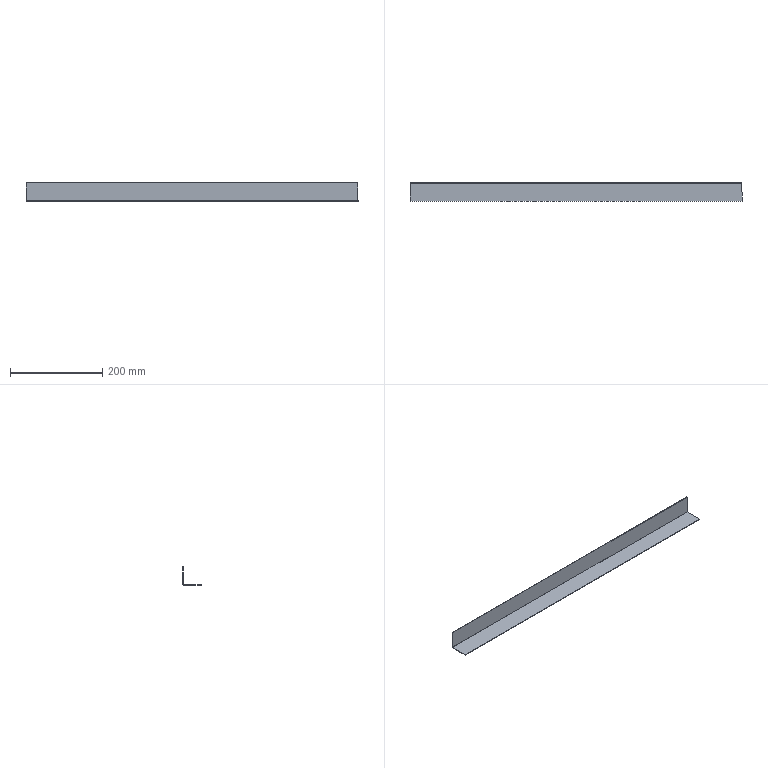Part | SolidWorks | features EdgeFlange 1, FlatPattern 1, SMBaseFlange 1, SheetMetal 1 | 1 solid | 14 faces | box 720 x 40 x 40 mm | volume 67824 mm3 | plane 12 | cylinder 2 | commonest cylinder face diameters 0.2 x1 2.6 x1
STEP:
#1=CARTESIAN_POINT('',(-360.,18.7,0.));
#2=VERTEX_POINT('',#1);
#3=CARTESIAN_POINT('',(-360.,-20.,0.));
#4=VERTEX_POINT('',#3);
#5=CARTESIAN_POINT('',(-360.,20.,0.));
#6=DIRECTION('',(0.,-1.,0.));
#7=VECTOR('',#6,1000.);
#8=LINE('',#5,#7);
#9=EDGE_CURVE('',#2,#4,#8,.T.);
#10=ORIENTED_EDGE('',*,*,#9,.F.);
#11=CARTESIAN_POINT('',(-360.,18.7,-1.2));
#12=VERTEX_POINT('',#11);
#13=CARTESIAN_POINT('',(-360.,18.7,0.));
#14=DIRECTION('',(0.,0.,-1.));
#15=VECTOR('',#14,1000.);
#16=LINE('',#13,#15);
#17=EDGE_CURVE('',#2,#12,#16,.T.);
#18=ORIENTED_EDGE('',*,*,#17,.T.);
#19=CARTESIAN_POINT('',(-360.,-20.,-1.2));
#20=VERTEX_POINT('',#19);
#21=CARTESIAN_POINT('',(-360.,20.,-1.2));
#22=DIRECTION('',(0.,-1.,0.));
#23=VECTOR('',#22,1000.);
#24=LINE('',#21,#23);
#25=EDGE_CURVE('',#12,#20,#24,.T.);
#26=ORIENTED_EDGE('',*,*,#25,.T.);
#27=CARTESIAN_POINT('',(-360.,-20.,-1.2));
#28=DIRECTION('',(0.,0.,1.));
#29=VECTOR('',#28,1000.);
#30=LINE('',#27,#29);
#31=EDGE_CURVE('',#20,#4,#30,.T.);
#32=ORIENTED_EDGE('',*,*,#31,.T.);
#33=EDGE_LOOP('',(#10,#18,#26,#32));
#34=FACE_OUTER_BOUND('',#33,.T.);
#35=CARTESIAN_POINT('',(-360.,20.,-1.2));
#36=DIRECTION('',(-1.,0.,0.));
#37=DIRECTION('',(0.,0.,1.));
#38=AXIS2_PLACEMENT_3D('',#35,#36,#37);
#39=PLANE('',#38);
#40=ADVANCED_FACE('',(#34),#39,.T.);
#41=CARTESIAN_POINT('',(360.,18.7,-1.2));
#42=VERTEX_POINT('',#41);
#43=CARTESIAN_POINT('',(-360.,18.7,-1.2));
#44=DIRECTION('',(1.,0.,0.));
#45=VECTOR('',#44,1000.);
#46=LINE('',#43,#45);
#47=EDGE_CURVE('',#12,#42,#46,.T.);
#48=ORIENTED_EDGE('',*,*,#47,.T.);
#49=CARTESIAN_POINT('',(360.,-20.,-1.2));
#50=VERTEX_POINT('',#49);
#51=CARTESIAN_POINT('',(360.,20.,-1.2));
#52=DIRECTION('',(0.,1.,0.));
#53=VECTOR('',#52,1000.);
#54=LINE('',#51,#53);
#55=EDGE_CURVE('',#50,#42,#54,.T.);
#56=ORIENTED_EDGE('',*,*,#55,.F.);
#57=CARTESIAN_POINT('',(-360.,-20.,-1.2));
#58=DIRECTION('',(1.,0.,0.));
#59=VECTOR('',#58,1000.);
#60=LINE('',#57,#59);
#61=EDGE_CURVE('',#20,#50,#60,.T.);
#62=ORIENTED_EDGE('',*,*,#61,.F.);
#63=ORIENTED_EDGE('',*,*,#25,.F.);
#64=EDGE_LOOP('',(#48,#56,#62,#63));
#65=FACE_OUTER_BOUND('',#64,.T.);
#66=CARTESIAN_POINT('',(0.,0.,-1.2));
#67=DIRECTION('',(0.,0.,1.));
#68=DIRECTION('',(1.,0.,0.));
#69=AXIS2_PLACEMENT_3D('',#66,#67,#68);
#70=PLANE('',#69);
#71=ADVANCED_FACE('',(#65),#70,.F.);
#72=CARTESIAN_POINT('',(360.,-20.,0.));
#73=VERTEX_POINT('',#72);
#74=CARTESIAN_POINT('',(360.,18.7,0.));
#75=VERTEX_POINT('',#74);
#76=CARTESIAN_POINT('',(360.,20.,0.));
#77=DIRECTION('',(0.,1.,0.));
#78=VECTOR('',#77,1000.);
#79=LINE('',#76,#78);
#80=EDGE_CURVE('',#73,#75,#79,.T.);
#81=ORIENTED_EDGE('',*,*,#80,.T.);
#82=CARTESIAN_POINT('',(-360.,18.7,0.));
#83=DIRECTION('',(1.,0.,0.));
#84=VECTOR('',#83,1000.);
#85=LINE('',#82,#84);
#86=EDGE_CURVE('',#2,#75,#85,.T.);
#87=ORIENTED_EDGE('',*,*,#86,.F.);
#88=ORIENTED_EDGE('',*,*,#9,.T.);
#89=CARTESIAN_POINT('',(-360.,-20.,0.));
#90=DIRECTION('',(1.,0.,0.));
#91=VECTOR('',#90,1000.);
#92=LINE('',#89,#91);
#93=EDGE_CURVE('',#4,#73,#92,.T.);
#94=ORIENTED_EDGE('',*,*,#93,.T.);
#95=EDGE_LOOP('',(#81,#87,#88,#94));
#96=FACE_OUTER_BOUND('',#95,.T.);
#97=CARTESIAN_POINT('',(0.,0.,0.));
#98=DIRECTION('',(0.,0.,1.));
#99=DIRECTION('',(1.,0.,0.));
#100=AXIS2_PLACEMENT_3D('',#97,#98,#99);
#101=PLANE('',#100);
#102=ADVANCED_FACE('',(#96),#101,.T.);
#103=CARTESIAN_POINT('',(360.,18.7,0.));
#104=DIRECTION('',(0.,0.,-1.));
#105=VECTOR('',#104,1000.);
#106=LINE('',#103,#105);
#107=EDGE_CURVE('',#75,#42,#106,.T.);
#108=ORIENTED_EDGE('',*,*,#107,.F.);
#109=ORIENTED_EDGE('',*,*,#80,.F.);
#110=CARTESIAN_POINT('',(360.,-20.,-1.2));
#111=DIRECTION('',(0.,0.,1.));
#112=VECTOR('',#111,1000.);
#113=LINE('',#110,#112);
#114=EDGE_CURVE('',#50,#73,#113,.T.);
#115=ORIENTED_EDGE('',*,*,#114,.F.);
#116=ORIENTED_EDGE('',*,*,#55,.T.);
#117=EDGE_LOOP('',(#108,#109,#115,#116));
#118=FACE_OUTER_BOUND('',#117,.T.);
#119=CARTESIAN_POINT('',(360.,20.,-1.2));
#120=DIRECTION('',(1.,0.,0.));
#121=DIRECTION('',(0.,0.,-1.));
#122=AXIS2_PLACEMENT_3D('',#119,#120,#121);
#123=PLANE('',#122);
#124=ADVANCED_FACE('',(#118),#123,.T.);
#125=ORIENTED_EDGE('',*,*,#93,.F.);
#126=ORIENTED_EDGE('',*,*,#31,.F.);
#127=ORIENTED_EDGE('',*,*,#61,.T.);
#128=ORIENTED_EDGE('',*,*,#114,.T.);
#129=EDGE_LOOP('',(#125,#126,#127,#128));
#130=FACE_OUTER_BOUND('',#129,.T.);
#131=CARTESIAN_POINT('',(-360.,-20.,-1.2));
#132=DIRECTION('',(0.,-1.,0.));
#133=DIRECTION('',(0.,0.,-1.));
#134=AXIS2_PLACEMENT_3D('',#131,#132,#133);
#135=PLANE('',#134);
#136=ADVANCED_FACE('',(#130),#135,.T.);
#137=CARTESIAN_POINT('',(360.,18.8,0.1));
#138=VERTEX_POINT('',#137);
#139=CARTESIAN_POINT('',(360.,20.,0.1));
#140=VERTEX_POINT('',#139);
#141=CARTESIAN_POINT('',(360.,20.,0.1));
#142=DIRECTION('',(0.,1.,0.));
#143=VECTOR('',#142,1000.);
#144=LINE('',#141,#143);
#145=EDGE_CURVE('',#138,#140,#144,.T.);
#146=ORIENTED_EDGE('',*,*,#145,.F.);
#147=CARTESIAN_POINT('',(360.,18.7,0.1));
#148=DIRECTION('',(1.,0.,0.));
#149=DIRECTION('',(0.,0.,1.));
#150=AXIS2_PLACEMENT_3D('',#147,#148,#149);
#151=CIRCLE('',#150,0.1);
#152=EDGE_CURVE('',#75,#138,#151,.T.);
#153=ORIENTED_EDGE('',*,*,#152,.F.);
#154=ORIENTED_EDGE('',*,*,#107,.T.);
#155=CARTESIAN_POINT('',(360.,18.7,0.1));
#156=DIRECTION('',(1.,0.,0.));
#157=DIRECTION('',(0.,0.,1.));
#158=AXIS2_PLACEMENT_3D('',#155,#156,#157);
#159=CIRCLE('',#158,1.3);
#160=EDGE_CURVE('',#42,#140,#159,.T.);
#161=ORIENTED_EDGE('',*,*,#160,.T.);
#162=EDGE_LOOP('',(#146,#153,#154,#161));
#163=FACE_OUTER_BOUND('',#162,.T.);
#164=CARTESIAN_POINT('',(360.,18.7,0.1));
#165=DIRECTION('',(1.,0.,0.));
#166=DIRECTION('',(0.,0.,-1.));
#167=AXIS2_PLACEMENT_3D('',#164,#165,#166);
#168=PLANE('',#167);
#169=ADVANCED_FACE('',(#163),#168,.T.);
#170=CARTESIAN_POINT('',(-360.,18.8,0.1));
#171=VERTEX_POINT('',#170);
#172=CARTESIAN_POINT('',(-360.,18.7,0.1));
#173=DIRECTION('',(-1.,0.,0.));
#174=DIRECTION('',(0.,0.,1.));
#175=AXIS2_PLACEMENT_3D('',#172,#173,#174);
#176=CIRCLE('',#175,0.1);
#177=EDGE_CURVE('',#171,#2,#176,.T.);
#178=ORIENTED_EDGE('',*,*,#177,.F.);
#179=CARTESIAN_POINT('',(-360.,20.,0.1));
#180=VERTEX_POINT('',#179);
#181=CARTESIAN_POINT('',(-360.,18.8,0.1));
#182=DIRECTION('',(0.,1.,0.));
#183=VECTOR('',#182,1000.);
#184=LINE('',#181,#183);
#185=EDGE_CURVE('',#171,#180,#184,.T.);
#186=ORIENTED_EDGE('',*,*,#185,.T.);
#187=CARTESIAN_POINT('',(-360.,18.7,0.1));
#188=DIRECTION('',(-1.,0.,0.));
#189=DIRECTION('',(0.,0.,1.));
#190=AXIS2_PLACEMENT_3D('',#187,#188,#189);
#191=CIRCLE('',#190,1.3);
#192=EDGE_CURVE('',#180,#12,#191,.T.);
#193=ORIENTED_EDGE('',*,*,#192,.T.);
#194=ORIENTED_EDGE('',*,*,#17,.F.);
#195=EDGE_LOOP('',(#178,#186,#193,#194));
#196=FACE_OUTER_BOUND('',#195,.T.);
#197=CARTESIAN_POINT('',(-360.,18.7,0.1));
#198=DIRECTION('',(1.,0.,0.));
#199=DIRECTION('',(0.,0.,-1.));
#200=AXIS2_PLACEMENT_3D('',#197,#198,#199);
#201=PLANE('',#200);
#202=ADVANCED_FACE('',(#196),#201,.F.);
#203=ORIENTED_EDGE('',*,*,#47,.F.);
#204=ORIENTED_EDGE('',*,*,#192,.F.);
#205=CARTESIAN_POINT('',(360.,20.,0.1));
#206=DIRECTION('',(1.,0.,0.));
#207=VECTOR('',#206,1000.);
#208=LINE('',#205,#207);
#209=EDGE_CURVE('',#180,#140,#208,.T.);
#210=ORIENTED_EDGE('',*,*,#209,.T.);
#211=ORIENTED_EDGE('',*,*,#160,.F.);
#212=EDGE_LOOP('',(#203,#204,#210,#211));
#213=FACE_OUTER_BOUND('',#212,.T.);
#214=CARTESIAN_POINT('',(-360.,18.7,0.1));
#215=DIRECTION('',(-1.,0.,0.));
#216=DIRECTION('',(0.,1.,0.));
#217=AXIS2_PLACEMENT_3D('',#214,#215,#216);
#218=CYLINDRICAL_SURFACE('',#217,1.3);
#219=ADVANCED_FACE('',(#213),#218,.T.);
#220=ORIENTED_EDGE('',*,*,#86,.T.);
#221=ORIENTED_EDGE('',*,*,#152,.T.);
#222=CARTESIAN_POINT('',(360.,18.8,0.1));
#223=DIRECTION('',(-1.,0.,0.));
#224=VECTOR('',#223,1000.);
#225=LINE('',#222,#224);
#226=EDGE_CURVE('',#138,#171,#225,.T.);
#227=ORIENTED_EDGE('',*,*,#226,.T.);
#228=ORIENTED_EDGE('',*,*,#177,.T.);
#229=EDGE_LOOP('',(#220,#221,#227,#228));
#230=FACE_OUTER_BOUND('',#229,.T.);
#231=CARTESIAN_POINT('',(-360.,18.7,0.1));
#232=DIRECTION('',(-1.,0.,0.));
#233=DIRECTION('',(0.,1.,0.));
#234=AXIS2_PLACEMENT_3D('',#231,#232,#233);
#235=CYLINDRICAL_SURFACE('',#234,0.1);
#236=ADVANCED_FACE('',(#230),#235,.F.);
#237=ORIENTED_EDGE('',*,*,#185,.F.);
#238=CARTESIAN_POINT('',(-360.,18.8,38.8));
#239=VERTEX_POINT('',#238);
#240=CARTESIAN_POINT('',(-360.,18.8,38.8));
#241=DIRECTION('',(0.,0.,1.));
#242=VECTOR('',#241,1000.);
#243=LINE('',#240,#242);
#244=EDGE_CURVE('',#171,#239,#243,.T.);
#245=ORIENTED_EDGE('',*,*,#244,.T.);
#246=CARTESIAN_POINT('',(-360.,20.,38.8));
#247=VERTEX_POINT('',#246);
#248=CARTESIAN_POINT('',(-360.,20.,38.8));
#249=DIRECTION('',(0.,-1.,0.));
#250=VECTOR('',#249,1000.);
#251=LINE('',#248,#250);
#252=EDGE_CURVE('',#247,#239,#251,.T.);
#253=ORIENTED_EDGE('',*,*,#252,.F.);
#254=CARTESIAN_POINT('',(-360.,20.,0.));
#255=DIRECTION('',(0.,0.,1.));
#256=VECTOR('',#255,1000.);
#257=LINE('',#254,#256);
#258=EDGE_CURVE('',#180,#247,#257,.T.);
#259=ORIENTED_EDGE('',*,*,#258,.F.);
#260=EDGE_LOOP('',(#237,#245,#253,#259));
#261=FACE_OUTER_BOUND('',#260,.T.);
#262=CARTESIAN_POINT('',(-360.,20.,38.8));
#263=DIRECTION('',(1.,0.,0.));
#264=DIRECTION('',(0.,0.,-1.));
#265=AXIS2_PLACEMENT_3D('',#262,#263,#264);
#266=PLANE('',#265);
#267=ADVANCED_FACE('',(#261),#266,.F.);
#268=ORIENTED_EDGE('',*,*,#145,.T.);
#269=CARTESIAN_POINT('',(360.,20.,38.8));
#270=VERTEX_POINT('',#269);
#271=CARTESIAN_POINT('',(360.,20.,0.));
#272=DIRECTION('',(0.,0.,-1.));
#273=VECTOR('',#272,1000.);
#274=LINE('',#271,#273);
#275=EDGE_CURVE('',#270,#140,#274,.T.);
#276=ORIENTED_EDGE('',*,*,#275,.F.);
#277=CARTESIAN_POINT('',(360.,18.8,38.8));
#278=VERTEX_POINT('',#277);
#279=CARTESIAN_POINT('',(360.,20.,38.8));
#280=DIRECTION('',(0.,-1.,0.));
#281=VECTOR('',#280,1000.);
#282=LINE('',#279,#281);
#283=EDGE_CURVE('',#270,#278,#282,.T.);
#284=ORIENTED_EDGE('',*,*,#283,.T.);
#285=CARTESIAN_POINT('',(360.,18.8,0.));
#286=DIRECTION('',(0.,0.,-1.));
#287=VECTOR('',#286,1000.);
#288=LINE('',#285,#287);
#289=EDGE_CURVE('',#278,#138,#288,.T.);
#290=ORIENTED_EDGE('',*,*,#289,.T.);
#291=EDGE_LOOP('',(#268,#276,#284,#290));
#292=FACE_OUTER_BOUND('',#291,.T.);
#293=CARTESIAN_POINT('',(360.,20.,0.));
#294=DIRECTION('',(-1.,0.,0.));
#295=DIRECTION('',(0.,0.,1.));
#296=AXIS2_PLACEMENT_3D('',#293,#294,#295);
#297=PLANE('',#296);
#298=ADVANCED_FACE('',(#292),#297,.F.);
#299=ORIENTED_EDGE('',*,*,#209,.F.);
#300=ORIENTED_EDGE('',*,*,#258,.T.);
#301=CARTESIAN_POINT('',(0.,20.,38.8));
#302=DIRECTION('',(1.,0.,0.));
#303=VECTOR('',#302,1000.);
#304=LINE('',#301,#303);
#305=EDGE_CURVE('',#247,#270,#304,.T.);
#306=ORIENTED_EDGE('',*,*,#305,.T.);
#307=ORIENTED_EDGE('',*,*,#275,.T.);
#308=EDGE_LOOP('',(#299,#300,#306,#307));
#309=FACE_OUTER_BOUND('',#308,.T.);
#310=CARTESIAN_POINT('',(0.,20.,0.));
#311=DIRECTION('',(0.,-1.,0.));
#312=DIRECTION('',(0.,0.,-1.));
#313=AXIS2_PLACEMENT_3D('',#310,#311,#312);
#314=PLANE('',#313);
#315=ADVANCED_FACE('',(#309),#314,.F.);
#316=ORIENTED_EDGE('',*,*,#244,.F.);
#317=ORIENTED_EDGE('',*,*,#226,.F.);
#318=ORIENTED_EDGE('',*,*,#289,.F.);
#319=CARTESIAN_POINT('',(360.,18.8,38.8));
#320=DIRECTION('',(1.,0.,0.));
#321=VECTOR('',#320,1000.);
#322=LINE('',#319,#321);
#323=EDGE_CURVE('',#239,#278,#322,.T.);
#324=ORIENTED_EDGE('',*,*,#323,.F.);
#325=EDGE_LOOP('',(#316,#317,#318,#324));
#326=FACE_OUTER_BOUND('',#325,.T.);
#327=CARTESIAN_POINT('',(0.,18.8,0.));
#328=DIRECTION('',(0.,-1.,0.));
#329=DIRECTION('',(0.,0.,-1.));
#330=AXIS2_PLACEMENT_3D('',#327,#328,#329);
#331=PLANE('',#330);
#332=ADVANCED_FACE('',(#326),#331,.T.);
#333=ORIENTED_EDGE('',*,*,#323,.T.);
#334=ORIENTED_EDGE('',*,*,#283,.F.);
#335=ORIENTED_EDGE('',*,*,#305,.F.);
#336=ORIENTED_EDGE('',*,*,#252,.T.);
#337=EDGE_LOOP('',(#333,#334,#335,#336));
#338=FACE_OUTER_BOUND('',#337,.T.);
#339=CARTESIAN_POINT('',(360.,20.,38.8));
#340=DIRECTION('',(0.,0.,-1.));
#341=DIRECTION('',(0.,1.,0.));
#342=AXIS2_PLACEMENT_3D('',#339,#340,#341);
#343=PLANE('',#342);
#344=ADVANCED_FACE('',(#338),#343,.F.);
#345=CLOSED_SHELL('',(#40,#71,#102,#124,#136,#169,#202,#219,#236,#267,#298,#315,#332,#344));
#346=MANIFOLD_SOLID_BREP('',#345);
#347=CARTESIAN_POINT('',(0.,0.,0.));
#348=DIRECTION('',(0.,0.,1.));
#349=DIRECTION('',(1.,0.,0.));
#350=AXIS2_PLACEMENT_3D('',#347,#348,#349);
#351=(LENGTH_UNIT()NAMED_UNIT(*)SI_UNIT(.MILLI.,.METRE.));
#352=UNCERTAINTY_MEASURE_WITH_UNIT(LENGTH_MEASURE(0.00001),#351,'','');
#353=(NAMED_UNIT(*)PLANE_ANGLE_UNIT()SI_UNIT($,.RADIAN.));
#354=(NAMED_UNIT(*)SI_UNIT($,.STERADIAN.)SOLID_ANGLE_UNIT());
#355=(GEOMETRIC_REPRESENTATION_CONTEXT(3)GLOBAL_UNCERTAINTY_ASSIGNED_CONTEXT((#352))GLOBAL_UNIT_ASSIGNED_CONTEXT((#351,#353,#354))REPRESENTATION_CONTEXT('',''));
#356=ADVANCED_BREP_SHAPE_REPRESENTATION('',(#346,#350),#355);